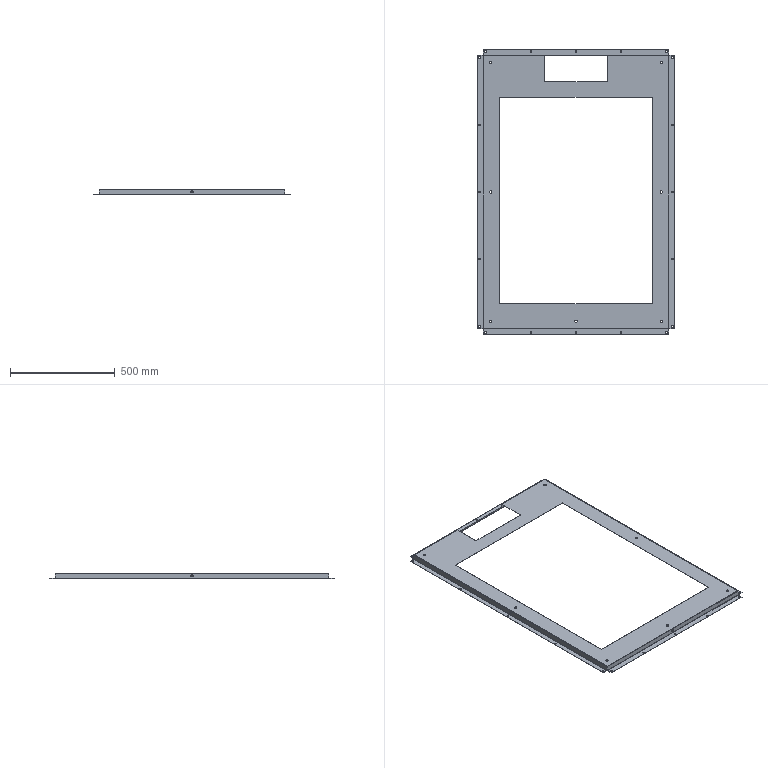Part | SolidWorks | features ICE 7, EdgeFlange 2, FlatPattern 1, SMBaseFlange 1, SheetMetal 1 | 1 solid | 194 faces | box 939 x 1359 x 25 mm | volume 613016 mm3 | plane 98 | cylinder 88 | spline 8 | commonest cylinder face diameters 7 x50 11 x14 0.4 x9 2.4 x9 10 x6